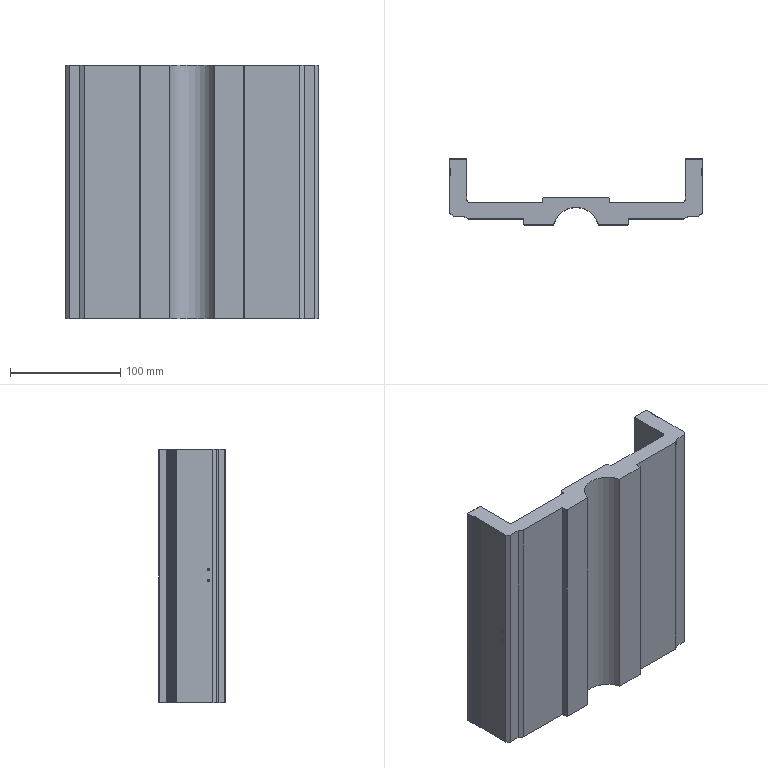Part | SolidWorks | features BaseBody 1 | 1 solid | 136 faces | box 230 x 60 x 230 mm | volume 1114980 mm3 | cylinder 63 | plane 49 | cone 24 | commonest cylinder face diameters 1 x28 6.8 x16 2.5 x8 2 x4 8 x4 4 x2